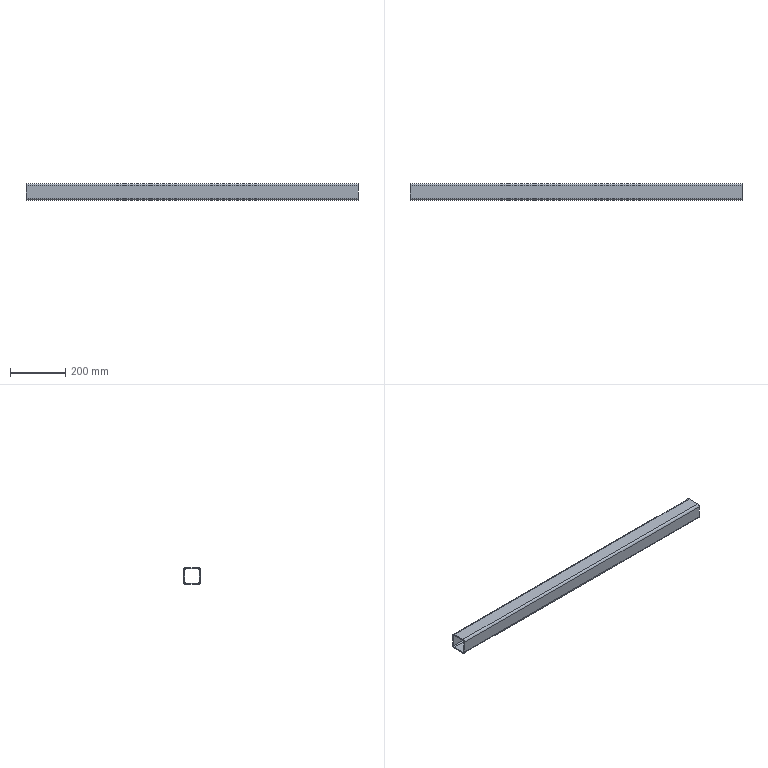Part | SolidWorks | features WeldMemberFeat 1, WeldmentFeature 1 | 1 solid | 18 faces | box 1200 x 60 x 60 mm | volume 1025756 mm3 | plane 10 | cylinder 8 | commonest cylinder face diameters 8 x4 16 x4
STEP:
#1=CARTESIAN_POINT('',(-600.,22.,-30.));
#2=VERTEX_POINT('',#1);
#3=CARTESIAN_POINT('',(-600.,30.,-22.));
#4=VERTEX_POINT('',#3);
#5=CARTESIAN_POINT('',(-600.,22.,-22.));
#6=DIRECTION('',(1.,0.,0.));
#7=DIRECTION('',(0.,0.,-1.));
#8=AXIS2_PLACEMENT_3D('',#5,#6,#7);
#9=CIRCLE('',#8,8.);
#10=EDGE_CURVE('',#2,#4,#9,.T.);
#11=ORIENTED_EDGE('',*,*,#10,.T.);
#12=CARTESIAN_POINT('',(600.,30.,-22.));
#13=VERTEX_POINT('',#12);
#14=CARTESIAN_POINT('',(600.,30.,-22.));
#15=DIRECTION('',(-1.,0.,0.));
#16=VECTOR('',#15,1000.);
#17=LINE('',#14,#16);
#18=EDGE_CURVE('',#13,#4,#17,.T.);
#19=ORIENTED_EDGE('',*,*,#18,.F.);
#20=CARTESIAN_POINT('',(600.,22.,-30.));
#21=VERTEX_POINT('',#20);
#22=CARTESIAN_POINT('',(600.,22.,-22.));
#23=DIRECTION('',(1.,0.,0.));
#24=DIRECTION('',(0.,0.,-1.));
#25=AXIS2_PLACEMENT_3D('',#22,#23,#24);
#26=CIRCLE('',#25,8.);
#27=EDGE_CURVE('',#21,#13,#26,.T.);
#28=ORIENTED_EDGE('',*,*,#27,.F.);
#29=CARTESIAN_POINT('',(600.,22.,-30.));
#30=DIRECTION('',(-1.,0.,0.));
#31=VECTOR('',#30,1000.);
#32=LINE('',#29,#31);
#33=EDGE_CURVE('',#21,#2,#32,.T.);
#34=ORIENTED_EDGE('',*,*,#33,.T.);
#35=EDGE_LOOP('',(#11,#19,#28,#34));
#36=FACE_OUTER_BOUND('',#35,.T.);
#37=CARTESIAN_POINT('',(600.,22.,-22.));
#38=DIRECTION('',(-1.,0.,0.));
#39=DIRECTION('',(0.,0.,1.));
#40=AXIS2_PLACEMENT_3D('',#37,#38,#39);
#41=CYLINDRICAL_SURFACE('',#40,8.);
#42=ADVANCED_FACE('',(#36),#41,.T.);
#43=CARTESIAN_POINT('',(-600.,30.,22.));
#44=VERTEX_POINT('',#43);
#45=CARTESIAN_POINT('',(-600.,30.,-22.));
#46=DIRECTION('',(0.,0.,1.));
#47=VECTOR('',#46,1000.);
#48=LINE('',#45,#47);
#49=EDGE_CURVE('',#4,#44,#48,.T.);
#50=ORIENTED_EDGE('',*,*,#49,.T.);
#51=CARTESIAN_POINT('',(600.,30.,22.));
#52=VERTEX_POINT('',#51);
#53=CARTESIAN_POINT('',(600.,30.,22.));
#54=DIRECTION('',(-1.,0.,0.));
#55=VECTOR('',#54,1000.);
#56=LINE('',#53,#55);
#57=EDGE_CURVE('',#52,#44,#56,.T.);
#58=ORIENTED_EDGE('',*,*,#57,.F.);
#59=CARTESIAN_POINT('',(600.,30.,-22.));
#60=DIRECTION('',(0.,0.,1.));
#61=VECTOR('',#60,1000.);
#62=LINE('',#59,#61);
#63=EDGE_CURVE('',#13,#52,#62,.T.);
#64=ORIENTED_EDGE('',*,*,#63,.F.);
#65=ORIENTED_EDGE('',*,*,#18,.T.);
#66=EDGE_LOOP('',(#50,#58,#64,#65));
#67=FACE_OUTER_BOUND('',#66,.T.);
#68=CARTESIAN_POINT('',(600.,30.,-22.));
#69=DIRECTION('',(0.,-1.,0.));
#70=DIRECTION('',(0.,0.,-1.));
#71=AXIS2_PLACEMENT_3D('',#68,#69,#70);
#72=PLANE('',#71);
#73=ADVANCED_FACE('',(#67),#72,.F.);
#74=CARTESIAN_POINT('',(-600.,22.,30.));
#75=VERTEX_POINT('',#74);
#76=CARTESIAN_POINT('',(-600.,22.,22.));
#77=DIRECTION('',(1.,0.,0.));
#78=DIRECTION('',(0.,0.,-1.));
#79=AXIS2_PLACEMENT_3D('',#76,#77,#78);
#80=CIRCLE('',#79,8.);
#81=EDGE_CURVE('',#44,#75,#80,.T.);
#82=ORIENTED_EDGE('',*,*,#81,.T.);
#83=CARTESIAN_POINT('',(600.,22.,30.));
#84=VERTEX_POINT('',#83);
#85=CARTESIAN_POINT('',(600.,22.,30.));
#86=DIRECTION('',(-1.,0.,0.));
#87=VECTOR('',#86,1000.);
#88=LINE('',#85,#87);
#89=EDGE_CURVE('',#84,#75,#88,.T.);
#90=ORIENTED_EDGE('',*,*,#89,.F.);
#91=CARTESIAN_POINT('',(600.,22.,22.));
#92=DIRECTION('',(1.,0.,0.));
#93=DIRECTION('',(0.,0.,-1.));
#94=AXIS2_PLACEMENT_3D('',#91,#92,#93);
#95=CIRCLE('',#94,8.);
#96=EDGE_CURVE('',#52,#84,#95,.T.);
#97=ORIENTED_EDGE('',*,*,#96,.F.);
#98=ORIENTED_EDGE('',*,*,#57,.T.);
#99=EDGE_LOOP('',(#82,#90,#97,#98));
#100=FACE_OUTER_BOUND('',#99,.T.);
#101=CARTESIAN_POINT('',(600.,22.,22.));
#102=DIRECTION('',(-1.,0.,0.));
#103=DIRECTION('',(0.,0.,1.));
#104=AXIS2_PLACEMENT_3D('',#101,#102,#103);
#105=CYLINDRICAL_SURFACE('',#104,8.);
#106=ADVANCED_FACE('',(#100),#105,.T.);
#107=CARTESIAN_POINT('',(-600.,-22.,30.));
#108=VERTEX_POINT('',#107);
#109=CARTESIAN_POINT('',(-600.,-22.,30.));
#110=DIRECTION('',(0.,-1.,0.));
#111=VECTOR('',#110,1000.);
#112=LINE('',#109,#111);
#113=EDGE_CURVE('',#75,#108,#112,.T.);
#114=ORIENTED_EDGE('',*,*,#113,.T.);
#115=CARTESIAN_POINT('',(600.,-22.,30.));
#116=VERTEX_POINT('',#115);
#117=CARTESIAN_POINT('',(600.,-22.,30.));
#118=DIRECTION('',(-1.,0.,0.));
#119=VECTOR('',#118,1000.);
#120=LINE('',#117,#119);
#121=EDGE_CURVE('',#116,#108,#120,.T.);
#122=ORIENTED_EDGE('',*,*,#121,.F.);
#123=CARTESIAN_POINT('',(600.,-22.,30.));
#124=DIRECTION('',(0.,-1.,0.));
#125=VECTOR('',#124,1000.);
#126=LINE('',#123,#125);
#127=EDGE_CURVE('',#84,#116,#126,.T.);
#128=ORIENTED_EDGE('',*,*,#127,.F.);
#129=ORIENTED_EDGE('',*,*,#89,.T.);
#130=EDGE_LOOP('',(#114,#122,#128,#129));
#131=FACE_OUTER_BOUND('',#130,.T.);
#132=CARTESIAN_POINT('',(600.,-22.,30.));
#133=DIRECTION('',(0.,0.,-1.));
#134=DIRECTION('',(-1.,0.,0.));
#135=AXIS2_PLACEMENT_3D('',#132,#133,#134);
#136=PLANE('',#135);
#137=ADVANCED_FACE('',(#131),#136,.F.);
#138=CARTESIAN_POINT('',(-600.,-30.,22.));
#139=VERTEX_POINT('',#138);
#140=CARTESIAN_POINT('',(-600.,-22.,22.));
#141=DIRECTION('',(1.,0.,0.));
#142=DIRECTION('',(0.,0.,-1.));
#143=AXIS2_PLACEMENT_3D('',#140,#141,#142);
#144=CIRCLE('',#143,8.);
#145=EDGE_CURVE('',#108,#139,#144,.T.);
#146=ORIENTED_EDGE('',*,*,#145,.T.);
#147=CARTESIAN_POINT('',(600.,-30.,22.));
#148=VERTEX_POINT('',#147);
#149=CARTESIAN_POINT('',(600.,-30.,22.));
#150=DIRECTION('',(-1.,0.,0.));
#151=VECTOR('',#150,1000.);
#152=LINE('',#149,#151);
#153=EDGE_CURVE('',#148,#139,#152,.T.);
#154=ORIENTED_EDGE('',*,*,#153,.F.);
#155=CARTESIAN_POINT('',(600.,-22.,22.));
#156=DIRECTION('',(1.,0.,0.));
#157=DIRECTION('',(0.,0.,-1.));
#158=AXIS2_PLACEMENT_3D('',#155,#156,#157);
#159=CIRCLE('',#158,8.);
#160=EDGE_CURVE('',#116,#148,#159,.T.);
#161=ORIENTED_EDGE('',*,*,#160,.F.);
#162=ORIENTED_EDGE('',*,*,#121,.T.);
#163=EDGE_LOOP('',(#146,#154,#161,#162));
#164=FACE_OUTER_BOUND('',#163,.T.);
#165=CARTESIAN_POINT('',(600.,-22.,22.));
#166=DIRECTION('',(-1.,0.,0.));
#167=DIRECTION('',(0.,0.,1.));
#168=AXIS2_PLACEMENT_3D('',#165,#166,#167);
#169=CYLINDRICAL_SURFACE('',#168,8.);
#170=ADVANCED_FACE('',(#164),#169,.T.);
#171=CARTESIAN_POINT('',(-600.,-30.,-22.));
#172=VERTEX_POINT('',#171);
#173=CARTESIAN_POINT('',(-600.,-30.,22.));
#174=DIRECTION('',(0.,0.,-1.));
#175=VECTOR('',#174,1000.);
#176=LINE('',#173,#175);
#177=EDGE_CURVE('',#139,#172,#176,.T.);
#178=ORIENTED_EDGE('',*,*,#177,.T.);
#179=CARTESIAN_POINT('',(600.,-30.,-22.));
#180=VERTEX_POINT('',#179);
#181=CARTESIAN_POINT('',(600.,-30.,-22.));
#182=DIRECTION('',(-1.,0.,0.));
#183=VECTOR('',#182,1000.);
#184=LINE('',#181,#183);
#185=EDGE_CURVE('',#180,#172,#184,.T.);
#186=ORIENTED_EDGE('',*,*,#185,.F.);
#187=CARTESIAN_POINT('',(600.,-30.,22.));
#188=DIRECTION('',(0.,0.,-1.));
#189=VECTOR('',#188,1000.);
#190=LINE('',#187,#189);
#191=EDGE_CURVE('',#148,#180,#190,.T.);
#192=ORIENTED_EDGE('',*,*,#191,.F.);
#193=ORIENTED_EDGE('',*,*,#153,.T.);
#194=EDGE_LOOP('',(#178,#186,#192,#193));
#195=FACE_OUTER_BOUND('',#194,.T.);
#196=CARTESIAN_POINT('',(600.,-30.,22.));
#197=DIRECTION('',(0.,1.,0.));
#198=DIRECTION('',(0.,0.,1.));
#199=AXIS2_PLACEMENT_3D('',#196,#197,#198);
#200=PLANE('',#199);
#201=ADVANCED_FACE('',(#195),#200,.F.);
#202=CARTESIAN_POINT('',(-600.,-22.,-30.));
#203=VERTEX_POINT('',#202);
#204=CARTESIAN_POINT('',(-600.,-22.,-22.));
#205=DIRECTION('',(1.,0.,0.));
#206=DIRECTION('',(0.,0.,-1.));
#207=AXIS2_PLACEMENT_3D('',#204,#205,#206);
#208=CIRCLE('',#207,8.);
#209=EDGE_CURVE('',#172,#203,#208,.T.);
#210=ORIENTED_EDGE('',*,*,#209,.T.);
#211=CARTESIAN_POINT('',(600.,-22.,-30.));
#212=VERTEX_POINT('',#211);
#213=CARTESIAN_POINT('',(600.,-22.,-30.));
#214=DIRECTION('',(-1.,0.,0.));
#215=VECTOR('',#214,1000.);
#216=LINE('',#213,#215);
#217=EDGE_CURVE('',#212,#203,#216,.T.);
#218=ORIENTED_EDGE('',*,*,#217,.F.);
#219=CARTESIAN_POINT('',(600.,-22.,-22.));
#220=DIRECTION('',(1.,0.,0.));
#221=DIRECTION('',(0.,0.,-1.));
#222=AXIS2_PLACEMENT_3D('',#219,#220,#221);
#223=CIRCLE('',#222,8.);
#224=EDGE_CURVE('',#180,#212,#223,.T.);
#225=ORIENTED_EDGE('',*,*,#224,.F.);
#226=ORIENTED_EDGE('',*,*,#185,.T.);
#227=EDGE_LOOP('',(#210,#218,#225,#226));
#228=FACE_OUTER_BOUND('',#227,.T.);
#229=CARTESIAN_POINT('',(600.,-22.,-22.));
#230=DIRECTION('',(-1.,0.,0.));
#231=DIRECTION('',(0.,0.,1.));
#232=AXIS2_PLACEMENT_3D('',#229,#230,#231);
#233=CYLINDRICAL_SURFACE('',#232,8.);
#234=ADVANCED_FACE('',(#228),#233,.T.);
#235=CARTESIAN_POINT('',(-600.,26.,22.));
#236=VERTEX_POINT('',#235);
#237=CARTESIAN_POINT('',(-600.,22.,26.));
#238=VERTEX_POINT('',#237);
#239=CARTESIAN_POINT('',(-600.,22.,22.));
#240=DIRECTION('',(1.,0.,0.));
#241=DIRECTION('',(0.,0.,-1.));
#242=AXIS2_PLACEMENT_3D('',#239,#240,#241);
#243=CIRCLE('',#242,4.);
#244=EDGE_CURVE('',#236,#238,#243,.T.);
#245=ORIENTED_EDGE('',*,*,#244,.F.);
#246=CARTESIAN_POINT('',(600.,26.,22.));
#247=VERTEX_POINT('',#246);
#248=CARTESIAN_POINT('',(600.,26.,22.));
#249=DIRECTION('',(-1.,0.,0.));
#250=VECTOR('',#249,1000.);
#251=LINE('',#248,#250);
#252=EDGE_CURVE('',#247,#236,#251,.T.);
#253=ORIENTED_EDGE('',*,*,#252,.F.);
#254=CARTESIAN_POINT('',(600.,22.,26.));
#255=VERTEX_POINT('',#254);
#256=CARTESIAN_POINT('',(600.,22.,22.));
#257=DIRECTION('',(1.,0.,0.));
#258=DIRECTION('',(0.,0.,-1.));
#259=AXIS2_PLACEMENT_3D('',#256,#257,#258);
#260=CIRCLE('',#259,4.);
#261=EDGE_CURVE('',#247,#255,#260,.T.);
#262=ORIENTED_EDGE('',*,*,#261,.T.);
#263=CARTESIAN_POINT('',(600.,22.,26.));
#264=DIRECTION('',(-1.,0.,0.));
#265=VECTOR('',#264,1000.);
#266=LINE('',#263,#265);
#267=EDGE_CURVE('',#255,#238,#266,.T.);
#268=ORIENTED_EDGE('',*,*,#267,.T.);
#269=EDGE_LOOP('',(#245,#253,#262,#268));
#270=FACE_OUTER_BOUND('',#269,.T.);
#271=CARTESIAN_POINT('',(600.,22.,22.));
#272=DIRECTION('',(-1.,0.,0.));
#273=DIRECTION('',(0.,0.,1.));
#274=AXIS2_PLACEMENT_3D('',#271,#272,#273);
#275=CYLINDRICAL_SURFACE('',#274,4.);
#276=ADVANCED_FACE('',(#270),#275,.F.);
#277=CARTESIAN_POINT('',(-600.,26.,-22.));
#278=VERTEX_POINT('',#277);
#279=CARTESIAN_POINT('',(-600.,26.,-22.));
#280=DIRECTION('',(0.,0.,1.));
#281=VECTOR('',#280,1000.);
#282=LINE('',#279,#281);
#283=EDGE_CURVE('',#278,#236,#282,.T.);
#284=ORIENTED_EDGE('',*,*,#283,.F.);
#285=CARTESIAN_POINT('',(600.,26.,-22.));
#286=VERTEX_POINT('',#285);
#287=CARTESIAN_POINT('',(600.,26.,-22.));
#288=DIRECTION('',(-1.,0.,0.));
#289=VECTOR('',#288,1000.);
#290=LINE('',#287,#289);
#291=EDGE_CURVE('',#286,#278,#290,.T.);
#292=ORIENTED_EDGE('',*,*,#291,.F.);
#293=CARTESIAN_POINT('',(600.,26.,-22.));
#294=DIRECTION('',(0.,0.,1.));
#295=VECTOR('',#294,1000.);
#296=LINE('',#293,#295);
#297=EDGE_CURVE('',#286,#247,#296,.T.);
#298=ORIENTED_EDGE('',*,*,#297,.T.);
#299=ORIENTED_EDGE('',*,*,#252,.T.);
#300=EDGE_LOOP('',(#284,#292,#298,#299));
#301=FACE_OUTER_BOUND('',#300,.T.);
#302=CARTESIAN_POINT('',(600.,26.,-22.));
#303=DIRECTION('',(0.,-1.,0.));
#304=DIRECTION('',(0.,0.,-1.));
#305=AXIS2_PLACEMENT_3D('',#302,#303,#304);
#306=PLANE('',#305);
#307=ADVANCED_FACE('',(#301),#306,.T.);
#308=CARTESIAN_POINT('',(-600.,22.,-26.));
#309=VERTEX_POINT('',#308);
#310=CARTESIAN_POINT('',(-600.,22.,-22.));
#311=DIRECTION('',(1.,0.,0.));
#312=DIRECTION('',(0.,0.,-1.));
#313=AXIS2_PLACEMENT_3D('',#310,#311,#312);
#314=CIRCLE('',#313,4.);
#315=EDGE_CURVE('',#309,#278,#314,.T.);
#316=ORIENTED_EDGE('',*,*,#315,.F.);
#317=CARTESIAN_POINT('',(600.,22.,-26.));
#318=VERTEX_POINT('',#317);
#319=CARTESIAN_POINT('',(600.,22.,-26.));
#320=DIRECTION('',(-1.,0.,0.));
#321=VECTOR('',#320,1000.);
#322=LINE('',#319,#321);
#323=EDGE_CURVE('',#318,#309,#322,.T.);
#324=ORIENTED_EDGE('',*,*,#323,.F.);
#325=CARTESIAN_POINT('',(600.,22.,-22.));
#326=DIRECTION('',(1.,0.,0.));
#327=DIRECTION('',(0.,0.,-1.));
#328=AXIS2_PLACEMENT_3D('',#325,#326,#327);
#329=CIRCLE('',#328,4.);
#330=EDGE_CURVE('',#318,#286,#329,.T.);
#331=ORIENTED_EDGE('',*,*,#330,.T.);
#332=ORIENTED_EDGE('',*,*,#291,.T.);
#333=EDGE_LOOP('',(#316,#324,#331,#332));
#334=FACE_OUTER_BOUND('',#333,.T.);
#335=CARTESIAN_POINT('',(600.,22.,-22.));
#336=DIRECTION('',(-1.,0.,0.));
#337=DIRECTION('',(0.,0.,1.));
#338=AXIS2_PLACEMENT_3D('',#335,#336,#337);
#339=CYLINDRICAL_SURFACE('',#338,4.);
#340=ADVANCED_FACE('',(#334),#339,.F.);
#341=CARTESIAN_POINT('',(-600.,-22.,-26.));
#342=VERTEX_POINT('',#341);
#343=CARTESIAN_POINT('',(-600.,22.,-26.));
#344=DIRECTION('',(0.,1.,0.));
#345=VECTOR('',#344,1000.);
#346=LINE('',#343,#345);
#347=EDGE_CURVE('',#342,#309,#346,.T.);
#348=ORIENTED_EDGE('',*,*,#347,.F.);
#349=CARTESIAN_POINT('',(600.,-22.,-26.));
#350=VERTEX_POINT('',#349);
#351=CARTESIAN_POINT('',(600.,-22.,-26.));
#352=DIRECTION('',(-1.,0.,0.));
#353=VECTOR('',#352,1000.);
#354=LINE('',#351,#353);
#355=EDGE_CURVE('',#350,#342,#354,.T.);
#356=ORIENTED_EDGE('',*,*,#355,.F.);
#357=CARTESIAN_POINT('',(600.,22.,-26.));
#358=DIRECTION('',(0.,1.,0.));
#359=VECTOR('',#358,1000.);
#360=LINE('',#357,#359);
#361=EDGE_CURVE('',#350,#318,#360,.T.);
#362=ORIENTED_EDGE('',*,*,#361,.T.);
#363=ORIENTED_EDGE('',*,*,#323,.T.);
#364=EDGE_LOOP('',(#348,#356,#362,#363));
#365=FACE_OUTER_BOUND('',#364,.T.);
#366=CARTESIAN_POINT('',(600.,22.,-26.));
#367=DIRECTION('',(0.,0.,1.));
#368=DIRECTION('',(1.,0.,0.));
#369=AXIS2_PLACEMENT_3D('',#366,#367,#368);
#370=PLANE('',#369);
#371=ADVANCED_FACE('',(#365),#370,.T.);
#372=CARTESIAN_POINT('',(-600.,-26.,-22.));
#373=VERTEX_POINT('',#372);
#374=CARTESIAN_POINT('',(-600.,-22.,-22.));
#375=DIRECTION('',(1.,0.,0.));
#376=DIRECTION('',(0.,0.,-1.));
#377=AXIS2_PLACEMENT_3D('',#374,#375,#376);
#378=CIRCLE('',#377,4.);
#379=EDGE_CURVE('',#373,#342,#378,.T.);
#380=ORIENTED_EDGE('',*,*,#379,.F.);
#381=CARTESIAN_POINT('',(600.,-26.,-22.));
#382=VERTEX_POINT('',#381);
#383=CARTESIAN_POINT('',(600.,-26.,-22.));
#384=DIRECTION('',(-1.,0.,0.));
#385=VECTOR('',#384,1000.);
#386=LINE('',#383,#385);
#387=EDGE_CURVE('',#382,#373,#386,.T.);
#388=ORIENTED_EDGE('',*,*,#387,.F.);
#389=CARTESIAN_POINT('',(600.,-22.,-22.));
#390=DIRECTION('',(1.,0.,0.));
#391=DIRECTION('',(0.,0.,-1.));
#392=AXIS2_PLACEMENT_3D('',#389,#390,#391);
#393=CIRCLE('',#392,4.);
#394=EDGE_CURVE('',#382,#350,#393,.T.);
#395=ORIENTED_EDGE('',*,*,#394,.T.);
#396=ORIENTED_EDGE('',*,*,#355,.T.);
#397=EDGE_LOOP('',(#380,#388,#395,#396));
#398=FACE_OUTER_BOUND('',#397,.T.);
#399=CARTESIAN_POINT('',(600.,-22.,-22.));
#400=DIRECTION('',(-1.,0.,0.));
#401=DIRECTION('',(0.,0.,1.));
#402=AXIS2_PLACEMENT_3D('',#399,#400,#401);
#403=CYLINDRICAL_SURFACE('',#402,4.);
#404=ADVANCED_FACE('',(#398),#403,.F.);
#405=CARTESIAN_POINT('',(-600.,-26.,22.));
#406=VERTEX_POINT('',#405);
#407=CARTESIAN_POINT('',(-600.,-26.,22.));
#408=DIRECTION('',(0.,0.,-1.));
#409=VECTOR('',#408,1000.);
#410=LINE('',#407,#409);
#411=EDGE_CURVE('',#406,#373,#410,.T.);
#412=ORIENTED_EDGE('',*,*,#411,.F.);
#413=CARTESIAN_POINT('',(600.,-26.,22.));
#414=VERTEX_POINT('',#413);
#415=CARTESIAN_POINT('',(600.,-26.,22.));
#416=DIRECTION('',(-1.,0.,0.));
#417=VECTOR('',#416,1000.);
#418=LINE('',#415,#417);
#419=EDGE_CURVE('',#414,#406,#418,.T.);
#420=ORIENTED_EDGE('',*,*,#419,.F.);
#421=CARTESIAN_POINT('',(600.,-26.,22.));
#422=DIRECTION('',(0.,0.,-1.));
#423=VECTOR('',#422,1000.);
#424=LINE('',#421,#423);
#425=EDGE_CURVE('',#414,#382,#424,.T.);
#426=ORIENTED_EDGE('',*,*,#425,.T.);
#427=ORIENTED_EDGE('',*,*,#387,.T.);
#428=EDGE_LOOP('',(#412,#420,#426,#427));
#429=FACE_OUTER_BOUND('',#428,.T.);
#430=CARTESIAN_POINT('',(600.,-26.,22.));
#431=DIRECTION('',(0.,1.,0.));
#432=DIRECTION('',(0.,0.,1.));
#433=AXIS2_PLACEMENT_3D('',#430,#431,#432);
#434=PLANE('',#433);
#435=ADVANCED_FACE('',(#429),#434,.T.);
#436=CARTESIAN_POINT('',(-600.,-22.,26.));
#437=VERTEX_POINT('',#436);
#438=CARTESIAN_POINT('',(-600.,-22.,22.));
#439=DIRECTION('',(1.,0.,0.));
#440=DIRECTION('',(0.,0.,-1.));
#441=AXIS2_PLACEMENT_3D('',#438,#439,#440);
#442=CIRCLE('',#441,4.);
#443=EDGE_CURVE('',#437,#406,#442,.T.);
#444=ORIENTED_EDGE('',*,*,#443,.F.);
#445=CARTESIAN_POINT('',(600.,-22.,26.));
#446=VERTEX_POINT('',#445);
#447=CARTESIAN_POINT('',(600.,-22.,26.));
#448=DIRECTION('',(-1.,0.,0.));
#449=VECTOR('',#448,1000.);
#450=LINE('',#447,#449);
#451=EDGE_CURVE('',#446,#437,#450,.T.);
#452=ORIENTED_EDGE('',*,*,#451,.F.);
#453=CARTESIAN_POINT('',(600.,-22.,22.));
#454=DIRECTION('',(1.,0.,0.));
#455=DIRECTION('',(0.,0.,-1.));
#456=AXIS2_PLACEMENT_3D('',#453,#454,#455);
#457=CIRCLE('',#456,4.);
#458=EDGE_CURVE('',#446,#414,#457,.T.);
#459=ORIENTED_EDGE('',*,*,#458,.T.);
#460=ORIENTED_EDGE('',*,*,#419,.T.);
#461=EDGE_LOOP('',(#444,#452,#459,#460));
#462=FACE_OUTER_BOUND('',#461,.T.);
#463=CARTESIAN_POINT('',(600.,-22.,22.));
#464=DIRECTION('',(-1.,0.,0.));
#465=DIRECTION('',(0.,0.,1.));
#466=AXIS2_PLACEMENT_3D('',#463,#464,#465);
#467=CYLINDRICAL_SURFACE('',#466,4.);
#468=ADVANCED_FACE('',(#462),#467,.F.);
#469=CARTESIAN_POINT('',(-600.,-22.,26.));
#470=DIRECTION('',(0.,-1.,0.));
#471=VECTOR('',#470,1000.);
#472=LINE('',#469,#471);
#473=EDGE_CURVE('',#238,#437,#472,.T.);
#474=ORIENTED_EDGE('',*,*,#473,.F.);
#475=ORIENTED_EDGE('',*,*,#267,.F.);
#476=CARTESIAN_POINT('',(600.,-22.,26.));
#477=DIRECTION('',(0.,-1.,0.));
#478=VECTOR('',#477,1000.);
#479=LINE('',#476,#478);
#480=EDGE_CURVE('',#255,#446,#479,.T.);
#481=ORIENTED_EDGE('',*,*,#480,.T.);
#482=ORIENTED_EDGE('',*,*,#451,.T.);
#483=EDGE_LOOP('',(#474,#475,#481,#482));
#484=FACE_OUTER_BOUND('',#483,.T.);
#485=CARTESIAN_POINT('',(600.,-22.,26.));
#486=DIRECTION('',(0.,0.,-1.));
#487=DIRECTION('',(-1.,0.,0.));
#488=AXIS2_PLACEMENT_3D('',#485,#486,#487);
#489=PLANE('',#488);
#490=ADVANCED_FACE('',(#484),#489,.T.);
#491=CARTESIAN_POINT('',(-600.,22.,-30.));
#492=DIRECTION('',(0.,1.,0.));
#493=VECTOR('',#492,1000.);
#494=LINE('',#491,#493);
#495=EDGE_CURVE('',#203,#2,#494,.T.);
#496=ORIENTED_EDGE('',*,*,#495,.T.);
#497=ORIENTED_EDGE('',*,*,#33,.F.);
#498=CARTESIAN_POINT('',(600.,22.,-30.));
#499=DIRECTION('',(0.,1.,0.));
#500=VECTOR('',#499,1000.);
#501=LINE('',#498,#500);
#502=EDGE_CURVE('',#212,#21,#501,.T.);
#503=ORIENTED_EDGE('',*,*,#502,.F.);
#504=ORIENTED_EDGE('',*,*,#217,.T.);
#505=EDGE_LOOP('',(#496,#497,#503,#504));
#506=FACE_OUTER_BOUND('',#505,.T.);
#507=CARTESIAN_POINT('',(600.,22.,-30.));
#508=DIRECTION('',(0.,0.,1.));
#509=DIRECTION('',(1.,0.,0.));
#510=AXIS2_PLACEMENT_3D('',#507,#508,#509);
#511=PLANE('',#510);
#512=ADVANCED_FACE('',(#506),#511,.F.);
#513=ORIENTED_EDGE('',*,*,#261,.F.);
#514=ORIENTED_EDGE('',*,*,#297,.F.);
#515=ORIENTED_EDGE('',*,*,#330,.F.);
#516=ORIENTED_EDGE('',*,*,#361,.F.);
#517=ORIENTED_EDGE('',*,*,#394,.F.);
#518=ORIENTED_EDGE('',*,*,#425,.F.);
#519=ORIENTED_EDGE('',*,*,#458,.F.);
#520=ORIENTED_EDGE('',*,*,#480,.F.);
#521=EDGE_LOOP('',(#513,#514,#515,#516,#517,#518,#519,#520));
#522=FACE_BOUND('',#521,.T.);
#523=ORIENTED_EDGE('',*,*,#27,.T.);
#524=ORIENTED_EDGE('',*,*,#63,.T.);
#525=ORIENTED_EDGE('',*,*,#96,.T.);
#526=ORIENTED_EDGE('',*,*,#127,.T.);
#527=ORIENTED_EDGE('',*,*,#160,.T.);
#528=ORIENTED_EDGE('',*,*,#191,.T.);
#529=ORIENTED_EDGE('',*,*,#224,.T.);
#530=ORIENTED_EDGE('',*,*,#502,.T.);
#531=EDGE_LOOP('',(#523,#524,#525,#526,#527,#528,#529,#530));
#532=FACE_OUTER_BOUND('',#531,.T.);
#533=CARTESIAN_POINT('',(600.,22.,-22.));
#534=DIRECTION('',(1.,0.,0.));
#535=DIRECTION('',(0.,0.,-1.));
#536=AXIS2_PLACEMENT_3D('',#533,#534,#535);
#537=PLANE('',#536);
#538=ADVANCED_FACE('',(#522,#532),#537,.T.);
#539=ORIENTED_EDGE('',*,*,#244,.T.);
#540=ORIENTED_EDGE('',*,*,#473,.T.);
#541=ORIENTED_EDGE('',*,*,#443,.T.);
#542=ORIENTED_EDGE('',*,*,#411,.T.);
#543=ORIENTED_EDGE('',*,*,#379,.T.);
#544=ORIENTED_EDGE('',*,*,#347,.T.);
#545=ORIENTED_EDGE('',*,*,#315,.T.);
#546=ORIENTED_EDGE('',*,*,#283,.T.);
#547=EDGE_LOOP('',(#539,#540,#541,#542,#543,#544,#545,#546));
#548=FACE_BOUND('',#547,.T.);
#549=ORIENTED_EDGE('',*,*,#10,.F.);
#550=ORIENTED_EDGE('',*,*,#495,.F.);
#551=ORIENTED_EDGE('',*,*,#209,.F.);
#552=ORIENTED_EDGE('',*,*,#177,.F.);
#553=ORIENTED_EDGE('',*,*,#145,.F.);
#554=ORIENTED_EDGE('',*,*,#113,.F.);
#555=ORIENTED_EDGE('',*,*,#81,.F.);
#556=ORIENTED_EDGE('',*,*,#49,.F.);
#557=EDGE_LOOP('',(#549,#550,#551,#552,#553,#554,#555,#556));
#558=FACE_OUTER_BOUND('',#557,.T.);
#559=CARTESIAN_POINT('',(-600.,22.,-22.));
#560=DIRECTION('',(1.,0.,0.));
#561=DIRECTION('',(0.,0.,-1.));
#562=AXIS2_PLACEMENT_3D('',#559,#560,#561);
#563=PLANE('',#562);
#564=ADVANCED_FACE('',(#548,#558),#563,.F.);
#565=CLOSED_SHELL('',(#42,#73,#106,#137,#170,#201,#234,#276,#307,#340,#371,#404,#435,#468,#490,#512,#538,#564));
#566=MANIFOLD_SOLID_BREP('',#565);
#567=CARTESIAN_POINT('',(0.,0.,0.));
#568=DIRECTION('',(0.,0.,1.));
#569=DIRECTION('',(1.,0.,0.));
#570=AXIS2_PLACEMENT_3D('',#567,#568,#569);
#571=(LENGTH_UNIT()NAMED_UNIT(*)SI_UNIT(.MILLI.,.METRE.));
#572=UNCERTAINTY_MEASURE_WITH_UNIT(LENGTH_MEASURE(0.00001),#571,'','');
#573=(NAMED_UNIT(*)PLANE_ANGLE_UNIT()SI_UNIT($,.RADIAN.));
#574=(NAMED_UNIT(*)SI_UNIT($,.STERADIAN.)SOLID_ANGLE_UNIT());
#575=(GEOMETRIC_REPRESENTATION_CONTEXT(3)GLOBAL_UNCERTAINTY_ASSIGNED_CONTEXT((#572))GLOBAL_UNIT_ASSIGNED_CONTEXT((#571,#573,#574))REPRESENTATION_CONTEXT('',''));
#576=ADVANCED_BREP_SHAPE_REPRESENTATION('',(#566,#570),#575);